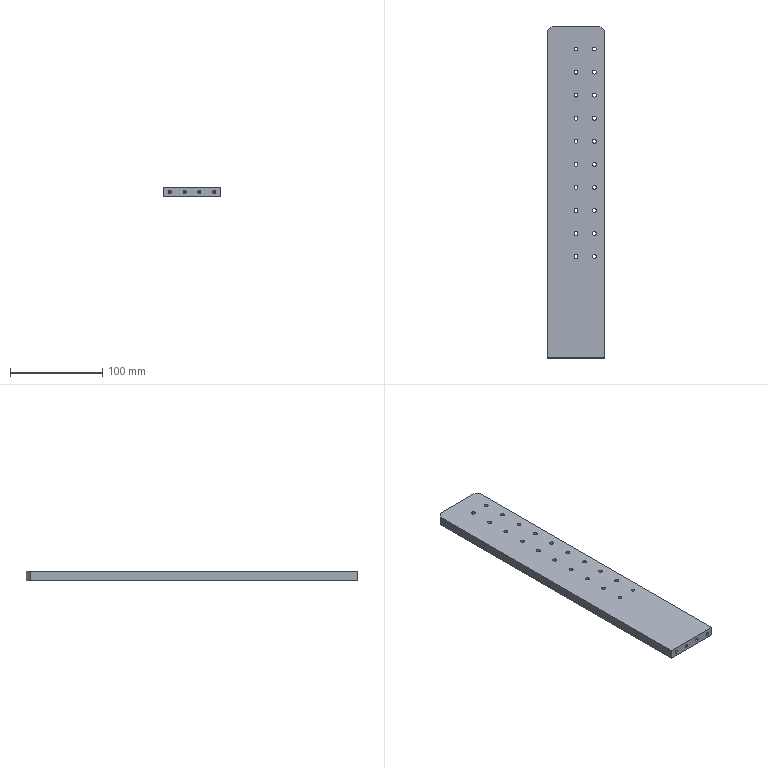Part | SolidWorks | features BaseBody 1 | 1 solid | 64 faces | box 62 x 360 x 10 mm | volume 219655 mm3 | cylinder 48 | cone 8 | plane 8 | commonest cylinder face diameters 4.2 x40 3.3 x8